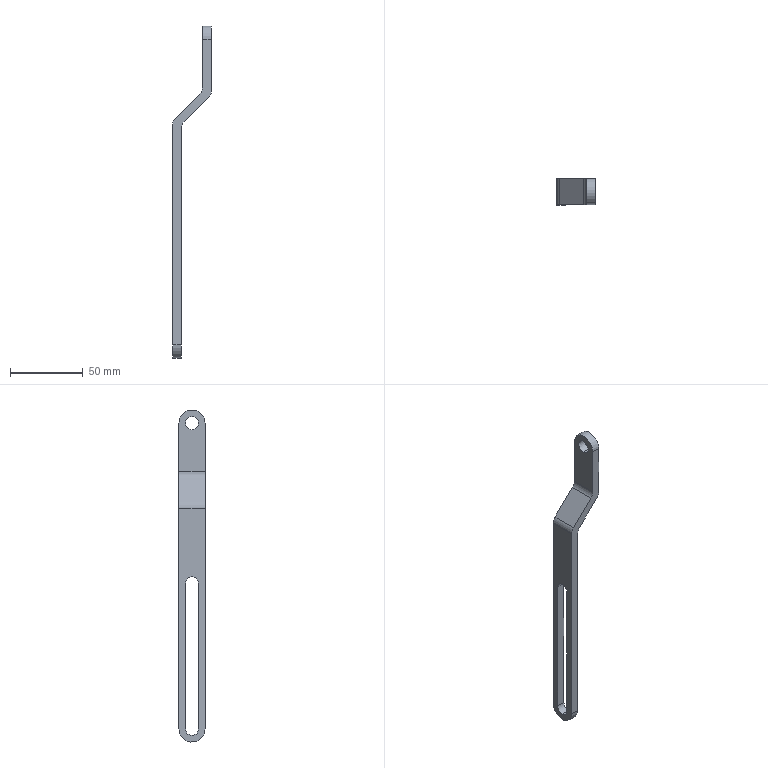Part | SolidWorks | features BaseBody 1 | 1 solid | 21 faces | box 26.5 x 18 x 228 mm | volume 18977 mm3 | cylinder 11 | plane 10 | commonest cylinder face diameters 9 x5 12 x4 18 x2
STEP:
#1=CARTESIAN_POINT('',(0.,13.5,-154.));
#2=VERTEX_POINT('',#1);
#3=CARTESIAN_POINT('',(0.,9.,-158.5));
#4=VERTEX_POINT('',#3);
#5=CARTESIAN_POINT('',(0.,9.,-154.));
#6=DIRECTION('',(-1.,0.,0.));
#7=DIRECTION('',(0.,0.,-1.));
#8=AXIS2_PLACEMENT_3D('',#5,#6,#7);
#9=CIRCLE('',#8,4.5);
#10=EDGE_CURVE('',#2,#4,#9,.T.);
#11=ORIENTED_EDGE('',*,*,#10,.T.);
#12=CARTESIAN_POINT('',(6.,9.,-158.5));
#13=VERTEX_POINT('',#12);
#14=CARTESIAN_POINT('',(0.,9.,-158.5));
#15=DIRECTION('',(1.,0.,0.));
#16=VECTOR('',#15,1000.);
#17=LINE('',#14,#16);
#18=EDGE_CURVE('',#4,#13,#17,.T.);
#19=ORIENTED_EDGE('',*,*,#18,.T.);
#20=CARTESIAN_POINT('',(6.,13.5,-154.));
#21=VERTEX_POINT('',#20);
#22=CARTESIAN_POINT('',(6.,9.,-154.));
#23=DIRECTION('',(-1.,0.,0.));
#24=DIRECTION('',(0.,0.,-1.));
#25=AXIS2_PLACEMENT_3D('',#22,#23,#24);
#26=CIRCLE('',#25,4.5);
#27=EDGE_CURVE('',#21,#13,#26,.T.);
#28=ORIENTED_EDGE('',*,*,#27,.F.);
#29=CARTESIAN_POINT('',(0.,13.5,-154.));
#30=DIRECTION('',(1.,0.,0.));
#31=VECTOR('',#30,1000.);
#32=LINE('',#29,#31);
#33=EDGE_CURVE('',#2,#21,#32,.T.);
#34=ORIENTED_EDGE('',*,*,#33,.F.);
#35=EDGE_LOOP('',(#11,#19,#28,#34));
#36=FACE_OUTER_BOUND('',#35,.T.);
#37=CARTESIAN_POINT('',(0.,9.,-154.));
#38=DIRECTION('',(1.,0.,0.));
#39=DIRECTION('',(0.,0.,-1.));
#40=AXIS2_PLACEMENT_3D('',#37,#38,#39);
#41=CYLINDRICAL_SURFACE('',#40,4.5);
#42=ADVANCED_FACE('',(#36),#41,.F.);
#43=CARTESIAN_POINT('',(20.5,9.,51.5));
#44=VERTEX_POINT('',#43);
#45=CARTESIAN_POINT('',(20.5,9.,60.5));
#46=VERTEX_POINT('',#45);
#47=CARTESIAN_POINT('',(20.5,9.,56.));
#48=DIRECTION('',(-1.,0.,0.));
#49=DIRECTION('',(0.,0.,-1.));
#50=AXIS2_PLACEMENT_3D('',#47,#48,#49);
#51=CIRCLE('',#50,4.5);
#52=EDGE_CURVE('',#44,#46,#51,.T.);
#53=ORIENTED_EDGE('',*,*,#52,.T.);
#54=CARTESIAN_POINT('',(26.5,9.,60.5));
#55=VERTEX_POINT('',#54);
#56=CARTESIAN_POINT('',(20.5,9.,60.5));
#57=DIRECTION('',(1.,0.,0.));
#58=VECTOR('',#57,1000.);
#59=LINE('',#56,#58);
#60=EDGE_CURVE('',#46,#55,#59,.T.);
#61=ORIENTED_EDGE('',*,*,#60,.T.);
#62=CARTESIAN_POINT('',(26.5,9.,51.5));
#63=VERTEX_POINT('',#62);
#64=CARTESIAN_POINT('',(26.5,9.,56.));
#65=DIRECTION('',(-1.,0.,0.));
#66=DIRECTION('',(0.,0.,-1.));
#67=AXIS2_PLACEMENT_3D('',#64,#65,#66);
#68=CIRCLE('',#67,4.5);
#69=EDGE_CURVE('',#63,#55,#68,.T.);
#70=ORIENTED_EDGE('',*,*,#69,.F.);
#71=CARTESIAN_POINT('',(20.5,9.,51.5));
#72=DIRECTION('',(1.,0.,0.));
#73=VECTOR('',#72,1000.);
#74=LINE('',#71,#73);
#75=EDGE_CURVE('',#44,#63,#74,.T.);
#76=ORIENTED_EDGE('',*,*,#75,.F.);
#77=EDGE_LOOP('',(#53,#61,#70,#76));
#78=FACE_OUTER_BOUND('',#77,.T.);
#79=CARTESIAN_POINT('',(20.5,9.,56.));
#80=DIRECTION('',(1.,0.,0.));
#81=DIRECTION('',(0.,0.,-1.));
#82=AXIS2_PLACEMENT_3D('',#79,#80,#81);
#83=CYLINDRICAL_SURFACE('',#82,4.5);
#84=ADVANCED_FACE('',(#78),#83,.F.);
#85=CARTESIAN_POINT('',(0.,4.5,-154.));
#86=VERTEX_POINT('',#85);
#87=CARTESIAN_POINT('',(0.,4.5,-54.));
#88=VERTEX_POINT('',#87);
#89=CARTESIAN_POINT('',(0.,4.5,-82.764));
#90=DIRECTION('',(0.,0.,1.));
#91=VECTOR('',#90,1000.);
#92=LINE('',#89,#91);
#93=EDGE_CURVE('',#86,#88,#92,.T.);
#94=ORIENTED_EDGE('',*,*,#93,.F.);
#95=CARTESIAN_POINT('',(0.,9.,-154.));
#96=DIRECTION('',(-1.,0.,0.));
#97=DIRECTION('',(0.,0.,-1.));
#98=AXIS2_PLACEMENT_3D('',#95,#96,#97);
#99=CIRCLE('',#98,4.5);
#100=EDGE_CURVE('',#4,#86,#99,.T.);
#101=ORIENTED_EDGE('',*,*,#100,.F.);
#102=ORIENTED_EDGE('',*,*,#10,.F.);
#103=CARTESIAN_POINT('',(0.,13.5,-54.));
#104=VERTEX_POINT('',#103);
#105=CARTESIAN_POINT('',(0.,13.5,-82.764));
#106=DIRECTION('',(0.,0.,-1.));
#107=VECTOR('',#106,1000.);
#108=LINE('',#105,#107);
#109=EDGE_CURVE('',#104,#2,#108,.T.);
#110=ORIENTED_EDGE('',*,*,#109,.F.);
#111=CARTESIAN_POINT('',(0.,9.,-54.));
#112=DIRECTION('',(-1.,0.,0.));
#113=DIRECTION('',(0.,0.,-1.));
#114=AXIS2_PLACEMENT_3D('',#111,#112,#113);
#115=CIRCLE('',#114,4.5);
#116=EDGE_CURVE('',#88,#104,#115,.T.);
#117=ORIENTED_EDGE('',*,*,#116,.F.);
#118=EDGE_LOOP('',(#94,#101,#102,#110,#117));
#119=FACE_BOUND('',#118,.T.);
#120=CARTESIAN_POINT('',(0.,18.,-154.));
#121=VERTEX_POINT('',#120);
#122=CARTESIAN_POINT('',(0.,18.,-2.529));
#123=VERTEX_POINT('',#122);
#124=CARTESIAN_POINT('',(0.,18.,-82.764));
#125=DIRECTION('',(0.,0.,1.));
#126=VECTOR('',#125,1000.);
#127=LINE('',#124,#126);
#128=EDGE_CURVE('',#121,#123,#127,.T.);
#129=ORIENTED_EDGE('',*,*,#128,.F.);
#130=CARTESIAN_POINT('',(0.,0.,-154.));
#131=VERTEX_POINT('',#130);
#132=CARTESIAN_POINT('',(0.,9.,-154.));
#133=DIRECTION('',(1.,0.,0.));
#134=DIRECTION('',(0.,0.,1.));
#135=AXIS2_PLACEMENT_3D('',#132,#133,#134);
#136=CIRCLE('',#135,9.);
#137=EDGE_CURVE('',#131,#121,#136,.T.);
#138=ORIENTED_EDGE('',*,*,#137,.F.);
#139=CARTESIAN_POINT('',(0.,0.,-2.529));
#140=VERTEX_POINT('',#139);
#141=CARTESIAN_POINT('',(0.,0.,-82.764));
#142=DIRECTION('',(0.,0.,-1.));
#143=VECTOR('',#142,1000.);
#144=LINE('',#141,#143);
#145=EDGE_CURVE('',#140,#131,#144,.T.);
#146=ORIENTED_EDGE('',*,*,#145,.F.);
#147=CARTESIAN_POINT('',(0.,9.,-2.529));
#148=DIRECTION('',(0.,-1.,0.));
#149=VECTOR('',#148,1000.);
#150=LINE('',#147,#149);
#151=EDGE_CURVE('',#123,#140,#150,.T.);
#152=ORIENTED_EDGE('',*,*,#151,.F.);
#153=EDGE_LOOP('',(#129,#138,#146,#152));
#154=FACE_OUTER_BOUND('',#153,.T.);
#155=CARTESIAN_POINT('',(0.,9.,-82.764));
#156=DIRECTION('',(1.,0.,0.));
#157=DIRECTION('',(0.,0.,-1.));
#158=AXIS2_PLACEMENT_3D('',#155,#156,#157);
#159=PLANE('',#158);
#160=ADVANCED_FACE('',(#119,#154),#159,.F.);
#161=CARTESIAN_POINT('',(6.,4.5,-54.));
#162=VERTEX_POINT('',#161);
#163=CARTESIAN_POINT('',(0.,4.5,-54.));
#164=DIRECTION('',(1.,0.,0.));
#165=VECTOR('',#164,1000.);
#166=LINE('',#163,#165);
#167=EDGE_CURVE('',#88,#162,#166,.T.);
#168=ORIENTED_EDGE('',*,*,#167,.F.);
#169=ORIENTED_EDGE('',*,*,#116,.T.);
#170=CARTESIAN_POINT('',(6.,13.5,-54.));
#171=VERTEX_POINT('',#170);
#172=CARTESIAN_POINT('',(0.,13.5,-54.));
#173=DIRECTION('',(-1.,0.,0.));
#174=VECTOR('',#173,1000.);
#175=LINE('',#172,#174);
#176=EDGE_CURVE('',#171,#104,#175,.T.);
#177=ORIENTED_EDGE('',*,*,#176,.F.);
#178=CARTESIAN_POINT('',(6.,9.,-54.));
#179=DIRECTION('',(-1.,0.,0.));
#180=DIRECTION('',(0.,0.,-1.));
#181=AXIS2_PLACEMENT_3D('',#178,#179,#180);
#182=CIRCLE('',#181,4.5);
#183=EDGE_CURVE('',#162,#171,#182,.T.);
#184=ORIENTED_EDGE('',*,*,#183,.F.);
#185=EDGE_LOOP('',(#168,#169,#177,#184));
#186=FACE_OUTER_BOUND('',#185,.T.);
#187=CARTESIAN_POINT('',(0.,9.,-54.));
#188=DIRECTION('',(1.,0.,0.));
#189=DIRECTION('',(0.,0.,-1.));
#190=AXIS2_PLACEMENT_3D('',#187,#188,#189);
#191=CYLINDRICAL_SURFACE('',#190,4.5);
#192=ADVANCED_FACE('',(#186),#191,.F.);
#193=CARTESIAN_POINT('',(6.,4.5,-154.));
#194=VERTEX_POINT('',#193);
#195=CARTESIAN_POINT('',(3.,4.5,-154.));
#196=DIRECTION('',(-1.,0.,0.));
#197=VECTOR('',#196,1000.);
#198=LINE('',#195,#197);
#199=EDGE_CURVE('',#194,#86,#198,.T.);
#200=ORIENTED_EDGE('',*,*,#199,.T.);
#201=ORIENTED_EDGE('',*,*,#93,.T.);
#202=ORIENTED_EDGE('',*,*,#167,.T.);
#203=CARTESIAN_POINT('',(6.,4.5,-104.));
#204=DIRECTION('',(0.,0.,-1.));
#205=VECTOR('',#204,1000.);
#206=LINE('',#203,#205);
#207=EDGE_CURVE('',#162,#194,#206,.T.);
#208=ORIENTED_EDGE('',*,*,#207,.T.);
#209=EDGE_LOOP('',(#200,#201,#202,#208));
#210=FACE_OUTER_BOUND('',#209,.T.);
#211=CARTESIAN_POINT('',(3.,4.5,-104.));
#212=DIRECTION('',(0.,1.,0.));
#213=DIRECTION('',(0.,0.,1.));
#214=AXIS2_PLACEMENT_3D('',#211,#212,#213);
#215=PLANE('',#214);
#216=ADVANCED_FACE('',(#210),#215,.T.);
#217=ORIENTED_EDGE('',*,*,#18,.F.);
#218=ORIENTED_EDGE('',*,*,#100,.T.);
#219=ORIENTED_EDGE('',*,*,#199,.F.);
#220=CARTESIAN_POINT('',(6.,9.,-154.));
#221=DIRECTION('',(-1.,0.,0.));
#222=DIRECTION('',(0.,0.,-1.));
#223=AXIS2_PLACEMENT_3D('',#220,#221,#222);
#224=CIRCLE('',#223,4.5);
#225=EDGE_CURVE('',#13,#194,#224,.T.);
#226=ORIENTED_EDGE('',*,*,#225,.F.);
#227=EDGE_LOOP('',(#217,#218,#219,#226));
#228=FACE_OUTER_BOUND('',#227,.T.);
#229=CARTESIAN_POINT('',(0.,9.,-154.));
#230=DIRECTION('',(1.,0.,0.));
#231=DIRECTION('',(0.,0.,-1.));
#232=AXIS2_PLACEMENT_3D('',#229,#230,#231);
#233=CYLINDRICAL_SURFACE('',#232,4.5);
#234=ADVANCED_FACE('',(#228),#233,.F.);
#235=CARTESIAN_POINT('',(6.,13.5,-104.));
#236=DIRECTION('',(0.,0.,-1.));
#237=VECTOR('',#236,1000.);
#238=LINE('',#235,#237);
#239=EDGE_CURVE('',#171,#21,#238,.T.);
#240=ORIENTED_EDGE('',*,*,#239,.F.);
#241=ORIENTED_EDGE('',*,*,#176,.T.);
#242=ORIENTED_EDGE('',*,*,#109,.T.);
#243=ORIENTED_EDGE('',*,*,#33,.T.);
#244=EDGE_LOOP('',(#240,#241,#242,#243));
#245=FACE_OUTER_BOUND('',#244,.T.);
#246=CARTESIAN_POINT('',(3.,13.5,-104.));
#247=DIRECTION('',(0.,1.,0.));
#248=DIRECTION('',(0.,0.,1.));
#249=AXIS2_PLACEMENT_3D('',#246,#247,#248);
#250=PLANE('',#249);
#251=ADVANCED_FACE('',(#245),#250,.F.);
#252=ORIENTED_EDGE('',*,*,#151,.T.);
#253=CARTESIAN_POINT('',(1.81,0.,1.766));
#254=VERTEX_POINT('',#253);
#255=CARTESIAN_POINT('',(6.,0.,-2.529));
#256=DIRECTION('',(0.,1.,0.));
#257=DIRECTION('',(0.,0.,-1.));
#258=AXIS2_PLACEMENT_3D('',#255,#256,#257);
#259=CIRCLE('',#258,6.);
#260=EDGE_CURVE('',#140,#254,#259,.T.);
#261=ORIENTED_EDGE('',*,*,#260,.T.);
#262=CARTESIAN_POINT('',(1.81,18.,1.766));
#263=VERTEX_POINT('',#262);
#264=CARTESIAN_POINT('',(1.81,18.,1.766));
#265=DIRECTION('',(0.,1.,0.));
#266=VECTOR('',#265,1000.);
#267=LINE('',#264,#266);
#268=EDGE_CURVE('',#254,#263,#267,.T.);
#269=ORIENTED_EDGE('',*,*,#268,.T.);
#270=CARTESIAN_POINT('',(6.,18.,-2.529));
#271=DIRECTION('',(0.,-1.,0.));
#272=DIRECTION('',(0.,0.,-1.));
#273=AXIS2_PLACEMENT_3D('',#270,#271,#272);
#274=CIRCLE('',#273,6.);
#275=EDGE_CURVE('',#263,#123,#274,.T.);
#276=ORIENTED_EDGE('',*,*,#275,.T.);
#277=EDGE_LOOP('',(#252,#261,#269,#276));
#278=FACE_OUTER_BOUND('',#277,.T.);
#279=CARTESIAN_POINT('',(6.,18.,-2.529));
#280=DIRECTION('',(0.,-1.,0.));
#281=DIRECTION('',(0.,0.,-1.));
#282=AXIS2_PLACEMENT_3D('',#279,#280,#281);
#283=CYLINDRICAL_SURFACE('',#282,6.);
#284=ADVANCED_FACE('',(#278),#283,.T.);
#285=ORIENTED_EDGE('',*,*,#275,.F.);
#286=CARTESIAN_POINT('',(18.69,18.,18.234));
#287=VERTEX_POINT('',#286);
#288=CARTESIAN_POINT('',(1.81,18.,1.766));
#289=DIRECTION('',(0.7158,0.,0.6983));
#290=VECTOR('',#289,1000.);
#291=LINE('',#288,#290);
#292=EDGE_CURVE('',#263,#287,#291,.T.);
#293=ORIENTED_EDGE('',*,*,#292,.T.);
#294=CARTESIAN_POINT('',(20.5,18.,22.529));
#295=VERTEX_POINT('',#294);
#296=CARTESIAN_POINT('',(14.5,18.,22.529));
#297=DIRECTION('',(0.,-1.,0.));
#298=DIRECTION('',(0.,0.,1.));
#299=AXIS2_PLACEMENT_3D('',#296,#297,#298);
#300=CIRCLE('',#299,6.);
#301=EDGE_CURVE('',#287,#295,#300,.T.);
#302=ORIENTED_EDGE('',*,*,#301,.T.);
#303=CARTESIAN_POINT('',(20.5,18.,56.));
#304=VERTEX_POINT('',#303);
#305=CARTESIAN_POINT('',(20.5,18.,-49.));
#306=DIRECTION('',(0.,0.,1.));
#307=VECTOR('',#306,1000.);
#308=LINE('',#305,#307);
#309=EDGE_CURVE('',#295,#304,#308,.T.);
#310=ORIENTED_EDGE('',*,*,#309,.T.);
#311=CARTESIAN_POINT('',(26.5,18.,56.));
#312=VERTEX_POINT('',#311);
#313=CARTESIAN_POINT('',(13.25,18.,56.));
#314=DIRECTION('',(1.,0.,0.));
#315=VECTOR('',#314,1000.);
#316=LINE('',#313,#315);
#317=EDGE_CURVE('',#304,#312,#316,.T.);
#318=ORIENTED_EDGE('',*,*,#317,.T.);
#319=CARTESIAN_POINT('',(26.5,18.,20.));
#320=VERTEX_POINT('',#319);
#321=CARTESIAN_POINT('',(26.5,18.,-49.));
#322=DIRECTION('',(0.,0.,-1.));
#323=VECTOR('',#322,1000.);
#324=LINE('',#321,#323);
#325=EDGE_CURVE('',#312,#320,#324,.T.);
#326=ORIENTED_EDGE('',*,*,#325,.T.);
#327=CARTESIAN_POINT('',(24.69,18.,15.705));
#328=VERTEX_POINT('',#327);
#329=CARTESIAN_POINT('',(20.5,18.,20.));
#330=DIRECTION('',(0.,1.,0.));
#331=DIRECTION('',(0.,0.,-1.));
#332=AXIS2_PLACEMENT_3D('',#329,#330,#331);
#333=CIRCLE('',#332,6.);
#334=EDGE_CURVE('',#320,#328,#333,.T.);
#335=ORIENTED_EDGE('',*,*,#334,.T.);
#336=CARTESIAN_POINT('',(7.81,18.,-0.7629));
#337=VERTEX_POINT('',#336);
#338=CARTESIAN_POINT('',(24.69,18.,15.705));
#339=DIRECTION('',(-0.7158,0.,-0.6983));
#340=VECTOR('',#339,1000.);
#341=LINE('',#338,#340);
#342=EDGE_CURVE('',#328,#337,#341,.T.);
#343=ORIENTED_EDGE('',*,*,#342,.T.);
#344=CARTESIAN_POINT('',(6.,18.,-5.058));
#345=VERTEX_POINT('',#344);
#346=CARTESIAN_POINT('',(12.,18.,-5.058));
#347=DIRECTION('',(0.,-1.,0.));
#348=DIRECTION('',(0.,0.,1.));
#349=AXIS2_PLACEMENT_3D('',#346,#347,#348);
#350=CIRCLE('',#349,6.);
#351=EDGE_CURVE('',#337,#345,#350,.T.);
#352=ORIENTED_EDGE('',*,*,#351,.T.);
#353=CARTESIAN_POINT('',(6.,18.,-154.));
#354=VERTEX_POINT('',#353);
#355=CARTESIAN_POINT('',(6.,18.,-49.));
#356=DIRECTION('',(0.,0.,-1.));
#357=VECTOR('',#356,1000.);
#358=LINE('',#355,#357);
#359=EDGE_CURVE('',#345,#354,#358,.T.);
#360=ORIENTED_EDGE('',*,*,#359,.T.);
#361=CARTESIAN_POINT('',(13.25,18.,-154.));
#362=DIRECTION('',(-1.,0.,0.));
#363=VECTOR('',#362,1000.);
#364=LINE('',#361,#363);
#365=EDGE_CURVE('',#354,#121,#364,.T.);
#366=ORIENTED_EDGE('',*,*,#365,.T.);
#367=ORIENTED_EDGE('',*,*,#128,.T.);
#368=EDGE_LOOP('',(#285,#293,#302,#310,#318,#326,#335,#343,#352,#360,#366,#367));
#369=FACE_OUTER_BOUND('',#368,.T.);
#370=CARTESIAN_POINT('',(13.25,18.,-49.));
#371=DIRECTION('',(0.,1.,0.));
#372=DIRECTION('',(0.,0.,1.));
#373=AXIS2_PLACEMENT_3D('',#370,#371,#372);
#374=PLANE('',#373);
#375=ADVANCED_FACE('',(#369),#374,.T.);
#376=CARTESIAN_POINT('',(6.,0.,-154.));
#377=VERTEX_POINT('',#376);
#378=CARTESIAN_POINT('',(6.,0.,-154.));
#379=DIRECTION('',(-1.,0.,0.));
#380=VECTOR('',#379,1000.);
#381=LINE('',#378,#380);
#382=EDGE_CURVE('',#377,#131,#381,.T.);
#383=ORIENTED_EDGE('',*,*,#382,.T.);
#384=ORIENTED_EDGE('',*,*,#137,.T.);
#385=ORIENTED_EDGE('',*,*,#365,.F.);
#386=CARTESIAN_POINT('',(6.,9.,-154.));
#387=DIRECTION('',(-1.,0.,0.));
#388=DIRECTION('',(0.,0.,1.));
#389=AXIS2_PLACEMENT_3D('',#386,#387,#388);
#390=CIRCLE('',#389,9.);
#391=EDGE_CURVE('',#354,#377,#390,.T.);
#392=ORIENTED_EDGE('',*,*,#391,.T.);
#393=EDGE_LOOP('',(#383,#384,#385,#392));
#394=FACE_OUTER_BOUND('',#393,.T.);
#395=CARTESIAN_POINT('',(6.,9.,-154.));
#396=DIRECTION('',(-1.,0.,0.));
#397=DIRECTION('',(0.,0.,1.));
#398=AXIS2_PLACEMENT_3D('',#395,#396,#397);
#399=CYLINDRICAL_SURFACE('',#398,9.);
#400=ADVANCED_FACE('',(#394),#399,.T.);
#401=ORIENTED_EDGE('',*,*,#260,.F.);
#402=ORIENTED_EDGE('',*,*,#145,.T.);
#403=ORIENTED_EDGE('',*,*,#382,.F.);
#404=CARTESIAN_POINT('',(6.,0.,-5.058));
#405=VERTEX_POINT('',#404);
#406=CARTESIAN_POINT('',(6.,0.,-49.));
#407=DIRECTION('',(0.,0.,-1.));
#408=VECTOR('',#407,1000.);
#409=LINE('',#406,#408);
#410=EDGE_CURVE('',#405,#377,#409,.T.);
#411=ORIENTED_EDGE('',*,*,#410,.F.);
#412=CARTESIAN_POINT('',(7.81,0.,-0.7629));
#413=VERTEX_POINT('',#412);
#414=CARTESIAN_POINT('',(12.,0.,-5.058));
#415=DIRECTION('',(0.,-1.,0.));
#416=DIRECTION('',(0.,0.,1.));
#417=AXIS2_PLACEMENT_3D('',#414,#415,#416);
#418=CIRCLE('',#417,6.);
#419=EDGE_CURVE('',#413,#405,#418,.T.);
#420=ORIENTED_EDGE('',*,*,#419,.F.);
#421=CARTESIAN_POINT('',(24.69,0.,15.705));
#422=VERTEX_POINT('',#421);
#423=CARTESIAN_POINT('',(24.69,0.,15.705));
#424=DIRECTION('',(-0.7158,0.,-0.6983));
#425=VECTOR('',#424,1000.);
#426=LINE('',#423,#425);
#427=EDGE_CURVE('',#422,#413,#426,.T.);
#428=ORIENTED_EDGE('',*,*,#427,.F.);
#429=CARTESIAN_POINT('',(26.5,0.,20.));
#430=VERTEX_POINT('',#429);
#431=CARTESIAN_POINT('',(20.5,0.,20.));
#432=DIRECTION('',(0.,1.,0.));
#433=DIRECTION('',(0.,0.,-1.));
#434=AXIS2_PLACEMENT_3D('',#431,#432,#433);
#435=CIRCLE('',#434,6.);
#436=EDGE_CURVE('',#430,#422,#435,.T.);
#437=ORIENTED_EDGE('',*,*,#436,.F.);
#438=CARTESIAN_POINT('',(26.5,0.,56.));
#439=VERTEX_POINT('',#438);
#440=CARTESIAN_POINT('',(26.5,0.,-49.));
#441=DIRECTION('',(0.,0.,-1.));
#442=VECTOR('',#441,1000.);
#443=LINE('',#440,#442);
#444=EDGE_CURVE('',#439,#430,#443,.T.);
#445=ORIENTED_EDGE('',*,*,#444,.F.);
#446=CARTESIAN_POINT('',(20.5,0.,56.));
#447=VERTEX_POINT('',#446);
#448=CARTESIAN_POINT('',(13.25,0.,56.));
#449=DIRECTION('',(1.,0.,0.));
#450=VECTOR('',#449,1000.);
#451=LINE('',#448,#450);
#452=EDGE_CURVE('',#447,#439,#451,.T.);
#453=ORIENTED_EDGE('',*,*,#452,.F.);
#454=CARTESIAN_POINT('',(20.5,0.,22.529));
#455=VERTEX_POINT('',#454);
#456=CARTESIAN_POINT('',(20.5,0.,-49.));
#457=DIRECTION('',(0.,0.,1.));
#458=VECTOR('',#457,1000.);
#459=LINE('',#456,#458);
#460=EDGE_CURVE('',#455,#447,#459,.T.);
#461=ORIENTED_EDGE('',*,*,#460,.F.);
#462=CARTESIAN_POINT('',(18.69,0.,18.234));
#463=VERTEX_POINT('',#462);
#464=CARTESIAN_POINT('',(14.5,0.,22.529));
#465=DIRECTION('',(0.,-1.,0.));
#466=DIRECTION('',(0.,0.,1.));
#467=AXIS2_PLACEMENT_3D('',#464,#465,#466);
#468=CIRCLE('',#467,6.);
#469=EDGE_CURVE('',#463,#455,#468,.T.);
#470=ORIENTED_EDGE('',*,*,#469,.F.);
#471=CARTESIAN_POINT('',(1.81,0.,1.766));
#472=DIRECTION('',(0.7158,0.,0.6983));
#473=VECTOR('',#472,1000.);
#474=LINE('',#471,#473);
#475=EDGE_CURVE('',#254,#463,#474,.T.);
#476=ORIENTED_EDGE('',*,*,#475,.F.);
#477=EDGE_LOOP('',(#401,#402,#403,#411,#420,#428,#437,#445,#453,#461,#470,#476));
#478=FACE_OUTER_BOUND('',#477,.T.);
#479=CARTESIAN_POINT('',(13.25,0.,-49.));
#480=DIRECTION('',(0.,1.,0.));
#481=DIRECTION('',(0.,0.,1.));
#482=AXIS2_PLACEMENT_3D('',#479,#480,#481);
#483=PLANE('',#482);
#484=ADVANCED_FACE('',(#478),#483,.F.);
#485=ORIENTED_EDGE('',*,*,#27,.T.);
#486=ORIENTED_EDGE('',*,*,#225,.T.);
#487=ORIENTED_EDGE('',*,*,#207,.F.);
#488=ORIENTED_EDGE('',*,*,#183,.T.);
#489=ORIENTED_EDGE('',*,*,#239,.T.);
#490=EDGE_LOOP('',(#485,#486,#487,#488,#489));
#491=FACE_BOUND('',#490,.T.);
#492=ORIENTED_EDGE('',*,*,#391,.F.);
#493=ORIENTED_EDGE('',*,*,#359,.F.);
#494=CARTESIAN_POINT('',(6.,9.,-5.058));
#495=DIRECTION('',(0.,-1.,0.));
#496=VECTOR('',#495,1000.);
#497=LINE('',#494,#496);
#498=EDGE_CURVE('',#345,#405,#497,.T.);
#499=ORIENTED_EDGE('',*,*,#498,.T.);
#500=ORIENTED_EDGE('',*,*,#410,.T.);
#501=EDGE_LOOP('',(#492,#493,#499,#500));
#502=FACE_OUTER_BOUND('',#501,.T.);
#503=CARTESIAN_POINT('',(6.,9.,-84.029));
#504=DIRECTION('',(1.,0.,0.));
#505=DIRECTION('',(0.,0.,-1.));
#506=AXIS2_PLACEMENT_3D('',#503,#504,#505);
#507=PLANE('',#506);
#508=ADVANCED_FACE('',(#491,#502),#507,.T.);
#509=ORIENTED_EDGE('',*,*,#268,.F.);
#510=ORIENTED_EDGE('',*,*,#475,.T.);
#511=CARTESIAN_POINT('',(18.69,9.,18.234));
#512=DIRECTION('',(0.,1.,0.));
#513=VECTOR('',#512,1000.);
#514=LINE('',#511,#513);
#515=EDGE_CURVE('',#463,#287,#514,.T.);
#516=ORIENTED_EDGE('',*,*,#515,.T.);
#517=ORIENTED_EDGE('',*,*,#292,.F.);
#518=EDGE_LOOP('',(#509,#510,#516,#517));
#519=FACE_OUTER_BOUND('',#518,.T.);
#520=CARTESIAN_POINT('',(10.25,9.,10.));
#521=DIRECTION('',(-0.6983,0.,0.7158));
#522=DIRECTION('',(0.7158,0.,0.6983));
#523=AXIS2_PLACEMENT_3D('',#520,#521,#522);
#524=PLANE('',#523);
#525=ADVANCED_FACE('',(#519),#524,.T.);
#526=ORIENTED_EDGE('',*,*,#351,.F.);
#527=CARTESIAN_POINT('',(7.81,0.,-0.7629));
#528=DIRECTION('',(0.,1.,0.));
#529=VECTOR('',#528,1000.);
#530=LINE('',#527,#529);
#531=EDGE_CURVE('',#413,#337,#530,.T.);
#532=ORIENTED_EDGE('',*,*,#531,.F.);
#533=ORIENTED_EDGE('',*,*,#419,.T.);
#534=ORIENTED_EDGE('',*,*,#498,.F.);
#535=EDGE_LOOP('',(#526,#532,#533,#534));
#536=FACE_OUTER_BOUND('',#535,.T.);
#537=CARTESIAN_POINT('',(12.,0.,-5.058));
#538=DIRECTION('',(0.,1.,0.));
#539=DIRECTION('',(0.,0.,1.));
#540=AXIS2_PLACEMENT_3D('',#537,#538,#539);
#541=CYLINDRICAL_SURFACE('',#540,6.);
#542=ADVANCED_FACE('',(#536),#541,.F.);
#543=ORIENTED_EDGE('',*,*,#342,.F.);
#544=CARTESIAN_POINT('',(24.69,9.,15.705));
#545=DIRECTION('',(0.,1.,0.));
#546=VECTOR('',#545,1000.);
#547=LINE('',#544,#546);
#548=EDGE_CURVE('',#422,#328,#547,.T.);
#549=ORIENTED_EDGE('',*,*,#548,.F.);
#550=ORIENTED_EDGE('',*,*,#427,.T.);
#551=ORIENTED_EDGE('',*,*,#531,.T.);
#552=EDGE_LOOP('',(#543,#549,#550,#551));
#553=FACE_OUTER_BOUND('',#552,.T.);
#554=CARTESIAN_POINT('',(16.25,9.,7.471));
#555=DIRECTION('',(-0.6983,0.,0.7158));
#556=DIRECTION('',(0.7158,0.,0.6983));
#557=AXIS2_PLACEMENT_3D('',#554,#555,#556);
#558=PLANE('',#557);
#559=ADVANCED_FACE('',(#553),#558,.F.);
#560=CARTESIAN_POINT('',(26.5,18.,20.));
#561=DIRECTION('',(0.,-1.,0.));
#562=VECTOR('',#561,1000.);
#563=LINE('',#560,#562);
#564=EDGE_CURVE('',#320,#430,#563,.T.);
#565=ORIENTED_EDGE('',*,*,#564,.T.);
#566=ORIENTED_EDGE('',*,*,#436,.T.);
#567=ORIENTED_EDGE('',*,*,#548,.T.);
#568=ORIENTED_EDGE('',*,*,#334,.F.);
#569=EDGE_LOOP('',(#565,#566,#567,#568));
#570=FACE_OUTER_BOUND('',#569,.T.);
#571=CARTESIAN_POINT('',(20.5,18.,20.));
#572=DIRECTION('',(0.,-1.,0.));
#573=DIRECTION('',(0.,0.,-1.));
#574=AXIS2_PLACEMENT_3D('',#571,#572,#573);
#575=CYLINDRICAL_SURFACE('',#574,6.);
#576=ADVANCED_FACE('',(#570),#575,.T.);
#577=ORIENTED_EDGE('',*,*,#69,.T.);
#578=CARTESIAN_POINT('',(26.5,9.,56.));
#579=DIRECTION('',(-1.,0.,0.));
#580=DIRECTION('',(0.,0.,-1.));
#581=AXIS2_PLACEMENT_3D('',#578,#579,#580);
#582=CIRCLE('',#581,4.5);
#583=EDGE_CURVE('',#55,#63,#582,.T.);
#584=ORIENTED_EDGE('',*,*,#583,.T.);
#585=EDGE_LOOP('',(#577,#584));
#586=FACE_BOUND('',#585,.T.);
#587=CARTESIAN_POINT('',(26.5,9.,56.));
#588=DIRECTION('',(1.,0.,0.));
#589=DIRECTION('',(0.,0.,-1.));
#590=AXIS2_PLACEMENT_3D('',#587,#588,#589);
#591=CIRCLE('',#590,9.);
#592=EDGE_CURVE('',#312,#439,#591,.T.);
#593=ORIENTED_EDGE('',*,*,#592,.T.);
#594=ORIENTED_EDGE('',*,*,#444,.T.);
#595=ORIENTED_EDGE('',*,*,#564,.F.);
#596=ORIENTED_EDGE('',*,*,#325,.F.);
#597=EDGE_LOOP('',(#593,#594,#595,#596));
#598=FACE_OUTER_BOUND('',#597,.T.);
#599=CARTESIAN_POINT('',(26.5,9.,42.5));
#600=DIRECTION('',(1.,0.,0.));
#601=DIRECTION('',(0.,0.,-1.));
#602=AXIS2_PLACEMENT_3D('',#599,#600,#601);
#603=PLANE('',#602);
#604=ADVANCED_FACE('',(#586,#598),#603,.T.);
#605=ORIENTED_EDGE('',*,*,#452,.T.);
#606=ORIENTED_EDGE('',*,*,#592,.F.);
#607=ORIENTED_EDGE('',*,*,#317,.F.);
#608=CARTESIAN_POINT('',(20.5,9.,56.));
#609=DIRECTION('',(1.,0.,0.));
#610=DIRECTION('',(0.,0.,-1.));
#611=AXIS2_PLACEMENT_3D('',#608,#609,#610);
#612=CIRCLE('',#611,9.);
#613=EDGE_CURVE('',#304,#447,#612,.T.);
#614=ORIENTED_EDGE('',*,*,#613,.T.);
#615=EDGE_LOOP('',(#605,#606,#607,#614));
#616=FACE_OUTER_BOUND('',#615,.T.);
#617=CARTESIAN_POINT('',(20.5,9.,56.));
#618=DIRECTION('',(1.,0.,0.));
#619=DIRECTION('',(0.,0.,-1.));
#620=AXIS2_PLACEMENT_3D('',#617,#618,#619);
#621=CYLINDRICAL_SURFACE('',#620,9.);
#622=ADVANCED_FACE('',(#616),#621,.T.);
#623=ORIENTED_EDGE('',*,*,#52,.F.);
#624=CARTESIAN_POINT('',(20.5,9.,56.));
#625=DIRECTION('',(-1.,0.,0.));
#626=DIRECTION('',(0.,0.,-1.));
#627=AXIS2_PLACEMENT_3D('',#624,#625,#626);
#628=CIRCLE('',#627,4.5);
#629=EDGE_CURVE('',#46,#44,#628,.T.);
#630=ORIENTED_EDGE('',*,*,#629,.F.);
#631=EDGE_LOOP('',(#623,#630));
#632=FACE_BOUND('',#631,.T.);
#633=ORIENTED_EDGE('',*,*,#460,.T.);
#634=ORIENTED_EDGE('',*,*,#613,.F.);
#635=ORIENTED_EDGE('',*,*,#309,.F.);
#636=CARTESIAN_POINT('',(20.5,9.,22.529));
#637=DIRECTION('',(0.,1.,0.));
#638=VECTOR('',#637,1000.);
#639=LINE('',#636,#638);
#640=EDGE_CURVE('',#455,#295,#639,.T.);
#641=ORIENTED_EDGE('',*,*,#640,.F.);
#642=EDGE_LOOP('',(#633,#634,#635,#641));
#643=FACE_OUTER_BOUND('',#642,.T.);
#644=CARTESIAN_POINT('',(20.5,9.,43.764));
#645=DIRECTION('',(1.,0.,0.));
#646=DIRECTION('',(0.,0.,-1.));
#647=AXIS2_PLACEMENT_3D('',#644,#645,#646);
#648=PLANE('',#647);
#649=ADVANCED_FACE('',(#632,#643),#648,.F.);
#650=ORIENTED_EDGE('',*,*,#301,.F.);
#651=ORIENTED_EDGE('',*,*,#515,.F.);
#652=ORIENTED_EDGE('',*,*,#469,.T.);
#653=ORIENTED_EDGE('',*,*,#640,.T.);
#654=EDGE_LOOP('',(#650,#651,#652,#653));
#655=FACE_OUTER_BOUND('',#654,.T.);
#656=CARTESIAN_POINT('',(14.5,0.,22.529));
#657=DIRECTION('',(0.,1.,0.));
#658=DIRECTION('',(0.,0.,1.));
#659=AXIS2_PLACEMENT_3D('',#656,#657,#658);
#660=CYLINDRICAL_SURFACE('',#659,6.);
#661=ADVANCED_FACE('',(#655),#660,.F.);
#662=ORIENTED_EDGE('',*,*,#60,.F.);
#663=ORIENTED_EDGE('',*,*,#629,.T.);
#664=ORIENTED_EDGE('',*,*,#75,.T.);
#665=ORIENTED_EDGE('',*,*,#583,.F.);
#666=EDGE_LOOP('',(#662,#663,#664,#665));
#667=FACE_OUTER_BOUND('',#666,.T.);
#668=CARTESIAN_POINT('',(20.5,9.,56.));
#669=DIRECTION('',(1.,0.,0.));
#670=DIRECTION('',(0.,0.,-1.));
#671=AXIS2_PLACEMENT_3D('',#668,#669,#670);
#672=CYLINDRICAL_SURFACE('',#671,4.5);
#673=ADVANCED_FACE('',(#667),#672,.F.);
#674=CLOSED_SHELL('',(#42,#84,#160,#192,#216,#234,#251,#284,#375,#400,#484,#508,#525,#542,#559,#576,#604,#622,#649,#661,#673));
#675=MANIFOLD_SOLID_BREP('',#674);
#676=CARTESIAN_POINT('',(0.,0.,0.));
#677=DIRECTION('',(0.,0.,1.));
#678=DIRECTION('',(1.,0.,0.));
#679=AXIS2_PLACEMENT_3D('',#676,#677,#678);
#680=(LENGTH_UNIT()NAMED_UNIT(*)SI_UNIT(.MILLI.,.METRE.));
#681=UNCERTAINTY_MEASURE_WITH_UNIT(LENGTH_MEASURE(0.00001),#680,'','');
#682=(NAMED_UNIT(*)PLANE_ANGLE_UNIT()SI_UNIT($,.RADIAN.));
#683=(NAMED_UNIT(*)SI_UNIT($,.STERADIAN.)SOLID_ANGLE_UNIT());
#684=(GEOMETRIC_REPRESENTATION_CONTEXT(3)GLOBAL_UNCERTAINTY_ASSIGNED_CONTEXT((#681))GLOBAL_UNIT_ASSIGNED_CONTEXT((#680,#682,#683))REPRESENTATION_CONTEXT('',''));
#685=ADVANCED_BREP_SHAPE_REPRESENTATION('',(#675,#679),#684);